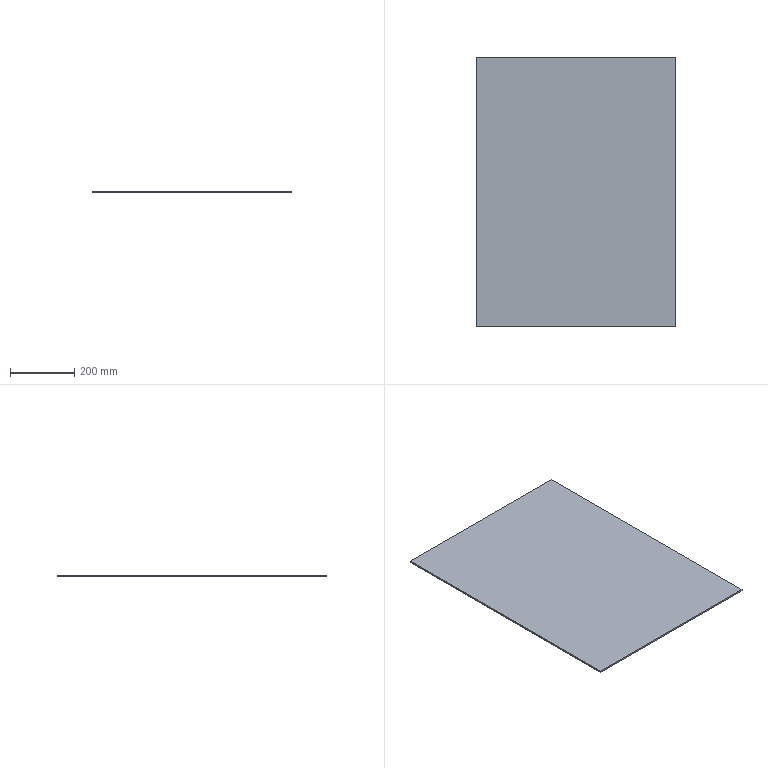Part | SolidWorks | features Extrusion 1, HoleWzd 1 | 1 solid | 6 faces | box 624 x 842 x 5 mm | volume 2627040 mm3 | plane 6
STEP:
#1=CARTESIAN_POINT('',(312.,-421.,0.));
#2=VERTEX_POINT('',#1);
#3=CARTESIAN_POINT('',(312.,421.,0.));
#4=VERTEX_POINT('',#3);
#5=CARTESIAN_POINT('',(312.,421.,0.));
#6=DIRECTION('',(0.,1.,0.));
#7=VECTOR('',#6,1000.);
#8=LINE('',#5,#7);
#9=EDGE_CURVE('',#2,#4,#8,.T.);
#10=ORIENTED_EDGE('',*,*,#9,.T.);
#11=CARTESIAN_POINT('',(312.,421.,5.));
#12=VERTEX_POINT('',#11);
#13=CARTESIAN_POINT('',(312.,421.,5.));
#14=DIRECTION('',(0.,0.,-1.));
#15=VECTOR('',#14,1000.);
#16=LINE('',#13,#15);
#17=EDGE_CURVE('',#12,#4,#16,.T.);
#18=ORIENTED_EDGE('',*,*,#17,.F.);
#19=CARTESIAN_POINT('',(312.,-421.,5.));
#20=VERTEX_POINT('',#19);
#21=CARTESIAN_POINT('',(312.,421.,5.));
#22=DIRECTION('',(0.,1.,0.));
#23=VECTOR('',#22,1000.);
#24=LINE('',#21,#23);
#25=EDGE_CURVE('',#20,#12,#24,.T.);
#26=ORIENTED_EDGE('',*,*,#25,.F.);
#27=CARTESIAN_POINT('',(312.,-421.,5.));
#28=DIRECTION('',(0.,0.,-1.));
#29=VECTOR('',#28,1000.);
#30=LINE('',#27,#29);
#31=EDGE_CURVE('',#20,#2,#30,.T.);
#32=ORIENTED_EDGE('',*,*,#31,.T.);
#33=EDGE_LOOP('',(#10,#18,#26,#32));
#34=FACE_OUTER_BOUND('',#33,.T.);
#35=CARTESIAN_POINT('',(312.,421.,5.));
#36=DIRECTION('',(-1.,0.,0.));
#37=DIRECTION('',(0.,-1.,0.));
#38=AXIS2_PLACEMENT_3D('',#35,#36,#37);
#39=PLANE('',#38);
#40=ADVANCED_FACE('',(#34),#39,.F.);
#41=CARTESIAN_POINT('',(-312.,421.,0.));
#42=VERTEX_POINT('',#41);
#43=CARTESIAN_POINT('',(-312.,421.,0.));
#44=DIRECTION('',(-1.,0.,0.));
#45=VECTOR('',#44,1000.);
#46=LINE('',#43,#45);
#47=EDGE_CURVE('',#4,#42,#46,.T.);
#48=ORIENTED_EDGE('',*,*,#47,.T.);
#49=CARTESIAN_POINT('',(-312.,421.,5.));
#50=VERTEX_POINT('',#49);
#51=CARTESIAN_POINT('',(-312.,421.,5.));
#52=DIRECTION('',(0.,0.,-1.));
#53=VECTOR('',#52,1000.);
#54=LINE('',#51,#53);
#55=EDGE_CURVE('',#50,#42,#54,.T.);
#56=ORIENTED_EDGE('',*,*,#55,.F.);
#57=CARTESIAN_POINT('',(-312.,421.,5.));
#58=DIRECTION('',(-1.,0.,0.));
#59=VECTOR('',#58,1000.);
#60=LINE('',#57,#59);
#61=EDGE_CURVE('',#12,#50,#60,.T.);
#62=ORIENTED_EDGE('',*,*,#61,.F.);
#63=ORIENTED_EDGE('',*,*,#17,.T.);
#64=EDGE_LOOP('',(#48,#56,#62,#63));
#65=FACE_OUTER_BOUND('',#64,.T.);
#66=CARTESIAN_POINT('',(-312.,421.,5.));
#67=DIRECTION('',(0.,-1.,0.));
#68=DIRECTION('',(0.,0.,-1.));
#69=AXIS2_PLACEMENT_3D('',#66,#67,#68);
#70=PLANE('',#69);
#71=ADVANCED_FACE('',(#65),#70,.F.);
#72=CARTESIAN_POINT('',(-312.,-421.,0.));
#73=VERTEX_POINT('',#72);
#74=CARTESIAN_POINT('',(-312.,421.,0.));
#75=DIRECTION('',(0.,-1.,0.));
#76=VECTOR('',#75,1000.);
#77=LINE('',#74,#76);
#78=EDGE_CURVE('',#42,#73,#77,.T.);
#79=ORIENTED_EDGE('',*,*,#78,.T.);
#80=CARTESIAN_POINT('',(-312.,-421.,5.));
#81=VERTEX_POINT('',#80);
#82=CARTESIAN_POINT('',(-312.,-421.,5.));
#83=DIRECTION('',(0.,0.,-1.));
#84=VECTOR('',#83,1000.);
#85=LINE('',#82,#84);
#86=EDGE_CURVE('',#81,#73,#85,.T.);
#87=ORIENTED_EDGE('',*,*,#86,.F.);
#88=CARTESIAN_POINT('',(-312.,421.,5.));
#89=DIRECTION('',(0.,-1.,0.));
#90=VECTOR('',#89,1000.);
#91=LINE('',#88,#90);
#92=EDGE_CURVE('',#50,#81,#91,.T.);
#93=ORIENTED_EDGE('',*,*,#92,.F.);
#94=ORIENTED_EDGE('',*,*,#55,.T.);
#95=EDGE_LOOP('',(#79,#87,#93,#94));
#96=FACE_OUTER_BOUND('',#95,.T.);
#97=CARTESIAN_POINT('',(-312.,421.,5.));
#98=DIRECTION('',(1.,0.,0.));
#99=DIRECTION('',(0.,1.,0.));
#100=AXIS2_PLACEMENT_3D('',#97,#98,#99);
#101=PLANE('',#100);
#102=ADVANCED_FACE('',(#96),#101,.F.);
#103=CARTESIAN_POINT('',(-312.,-421.,0.));
#104=DIRECTION('',(1.,0.,0.));
#105=VECTOR('',#104,1000.);
#106=LINE('',#103,#105);
#107=EDGE_CURVE('',#73,#2,#106,.T.);
#108=ORIENTED_EDGE('',*,*,#107,.T.);
#109=ORIENTED_EDGE('',*,*,#31,.F.);
#110=CARTESIAN_POINT('',(-312.,-421.,5.));
#111=DIRECTION('',(1.,0.,0.));
#112=VECTOR('',#111,1000.);
#113=LINE('',#110,#112);
#114=EDGE_CURVE('',#81,#20,#113,.T.);
#115=ORIENTED_EDGE('',*,*,#114,.F.);
#116=ORIENTED_EDGE('',*,*,#86,.T.);
#117=EDGE_LOOP('',(#108,#109,#115,#116));
#118=FACE_OUTER_BOUND('',#117,.T.);
#119=CARTESIAN_POINT('',(-312.,-421.,5.));
#120=DIRECTION('',(0.,1.,0.));
#121=DIRECTION('',(0.,0.,1.));
#122=AXIS2_PLACEMENT_3D('',#119,#120,#121);
#123=PLANE('',#122);
#124=ADVANCED_FACE('',(#118),#123,.F.);
#125=ORIENTED_EDGE('',*,*,#25,.T.);
#126=ORIENTED_EDGE('',*,*,#61,.T.);
#127=ORIENTED_EDGE('',*,*,#92,.T.);
#128=ORIENTED_EDGE('',*,*,#114,.T.);
#129=EDGE_LOOP('',(#125,#126,#127,#128));
#130=FACE_OUTER_BOUND('',#129,.T.);
#131=CARTESIAN_POINT('',(0.,0.,5.));
#132=DIRECTION('',(0.,0.,1.));
#133=DIRECTION('',(1.,0.,0.));
#134=AXIS2_PLACEMENT_3D('',#131,#132,#133);
#135=PLANE('',#134);
#136=ADVANCED_FACE('',(#130),#135,.T.);
#137=ORIENTED_EDGE('',*,*,#9,.F.);
#138=ORIENTED_EDGE('',*,*,#107,.F.);
#139=ORIENTED_EDGE('',*,*,#78,.F.);
#140=ORIENTED_EDGE('',*,*,#47,.F.);
#141=EDGE_LOOP('',(#137,#138,#139,#140));
#142=FACE_OUTER_BOUND('',#141,.T.);
#143=CARTESIAN_POINT('',(0.,0.,0.));
#144=DIRECTION('',(0.,0.,1.));
#145=DIRECTION('',(1.,0.,0.));
#146=AXIS2_PLACEMENT_3D('',#143,#144,#145);
#147=PLANE('',#146);
#148=ADVANCED_FACE('',(#142),#147,.F.);
#149=CLOSED_SHELL('',(#40,#71,#102,#124,#136,#148));
#150=MANIFOLD_SOLID_BREP('',#149);
#151=CARTESIAN_POINT('',(0.,0.,0.));
#152=DIRECTION('',(0.,0.,1.));
#153=DIRECTION('',(1.,0.,0.));
#154=AXIS2_PLACEMENT_3D('',#151,#152,#153);
#155=(LENGTH_UNIT()NAMED_UNIT(*)SI_UNIT(.MILLI.,.METRE.));
#156=UNCERTAINTY_MEASURE_WITH_UNIT(LENGTH_MEASURE(0.00001),#155,'','');
#157=(NAMED_UNIT(*)PLANE_ANGLE_UNIT()SI_UNIT($,.RADIAN.));
#158=(NAMED_UNIT(*)SI_UNIT($,.STERADIAN.)SOLID_ANGLE_UNIT());
#159=(GEOMETRIC_REPRESENTATION_CONTEXT(3)GLOBAL_UNCERTAINTY_ASSIGNED_CONTEXT((#156))GLOBAL_UNIT_ASSIGNED_CONTEXT((#155,#157,#158))REPRESENTATION_CONTEXT('',''));
#160=ADVANCED_BREP_SHAPE_REPRESENTATION('',(#150,#154),#159);